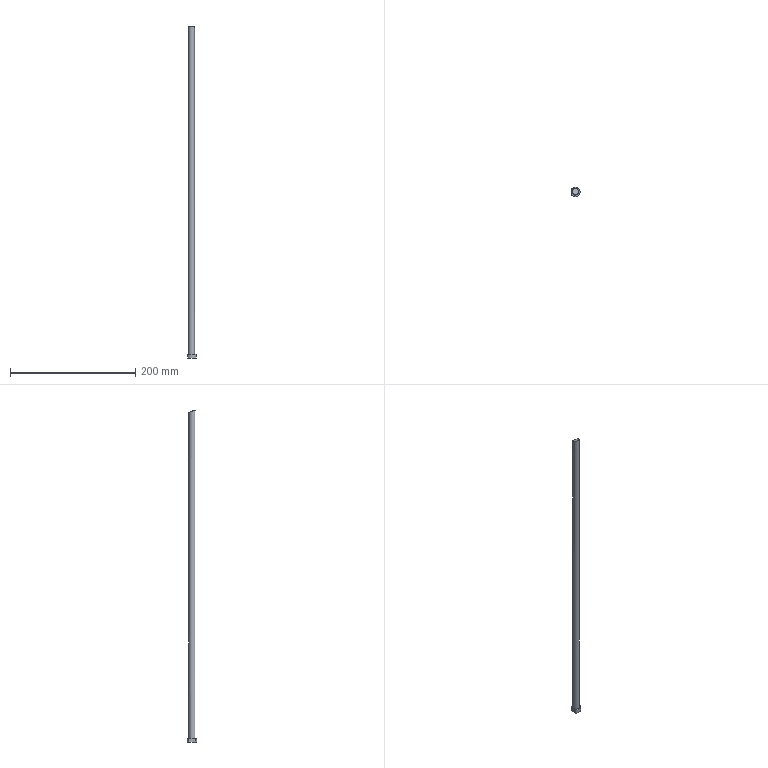Part | STEP file | solid 17 | 1 solid | 6 faces | box 13 x 15 x 530.22 mm | volume 41997 mm3 | plane 4 | cylinder 2 | commonest cylinder face diameters 10 x1 15 x1